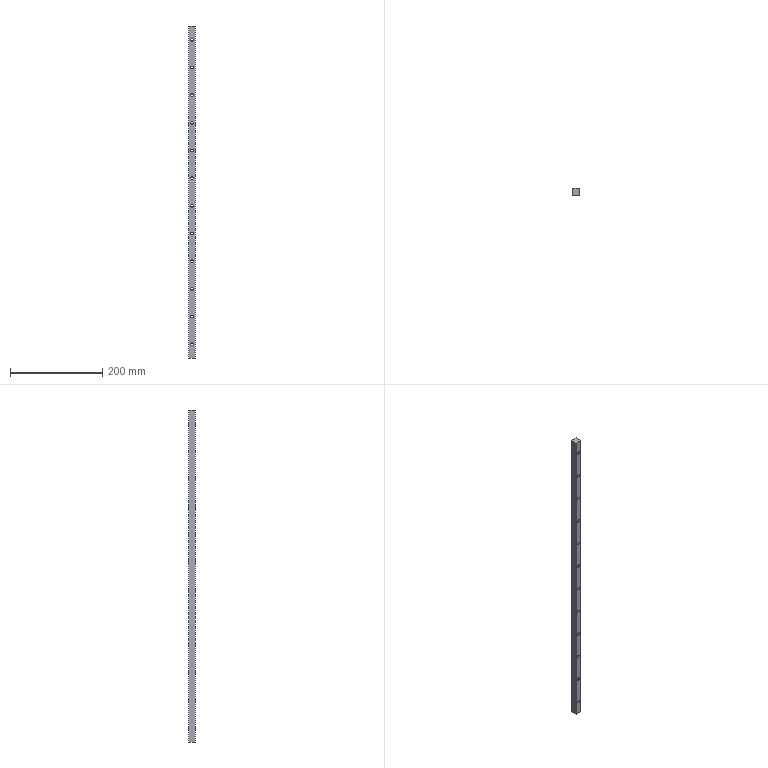Part | 1 solid | 30 faces | box 15 x 15 x 720 mm | volume 156911 mm3 | cylinder 24 | plane 6 | commonest cylinder face diameters 6 x24
STEP:
#1=CARTESIAN_POINT('',(7.5,0.,687.));
#2=VERTEX_POINT('',#1);
#3=CARTESIAN_POINT('',(7.5,0.,693.));
#4=VERTEX_POINT('',#3);
#5=CARTESIAN_POINT('',(7.5,0.,690.));
#6=DIRECTION('',(0.,1.,0.));
#7=DIRECTION('',(0.,0.,1.));
#8=AXIS2_PLACEMENT_3D('',#5,#6,#7);
#9=CIRCLE('',#8,3.);
#10=EDGE_CURVE('',#2,#4,#9,.T.);
#11=ORIENTED_EDGE('',*,*,#10,.F.);
#12=CARTESIAN_POINT('',(7.5,15.,687.));
#13=VERTEX_POINT('',#12);
#14=CARTESIAN_POINT('',(7.5,-35.,687.));
#15=DIRECTION('',(0.,1.,0.));
#16=VECTOR('',#15,1000.);
#17=LINE('',#14,#16);
#18=EDGE_CURVE('',#2,#13,#17,.T.);
#19=ORIENTED_EDGE('',*,*,#18,.T.);
#20=CARTESIAN_POINT('',(7.5,15.,693.));
#21=VERTEX_POINT('',#20);
#22=CARTESIAN_POINT('',(7.5,15.,690.));
#23=DIRECTION('',(0.,1.,0.));
#24=DIRECTION('',(0.,0.,1.));
#25=AXIS2_PLACEMENT_3D('',#22,#23,#24);
#26=CIRCLE('',#25,3.);
#27=EDGE_CURVE('',#13,#21,#26,.T.);
#28=ORIENTED_EDGE('',*,*,#27,.T.);
#29=CARTESIAN_POINT('',(7.5,-35.,693.));
#30=DIRECTION('',(0.,1.,0.));
#31=VECTOR('',#30,1000.);
#32=LINE('',#29,#31);
#33=EDGE_CURVE('',#4,#21,#32,.T.);
#34=ORIENTED_EDGE('',*,*,#33,.F.);
#35=EDGE_LOOP('',(#11,#19,#28,#34));
#36=FACE_OUTER_BOUND('',#35,.T.);
#37=CARTESIAN_POINT('',(7.5,-35.,690.));
#38=DIRECTION('',(0.,1.,0.));
#39=DIRECTION('',(0.,0.,1.));
#40=AXIS2_PLACEMENT_3D('',#37,#38,#39);
#41=CYLINDRICAL_SURFACE('',#40,3.);
#42=ADVANCED_FACE('',(#36),#41,.F.);
#43=CARTESIAN_POINT('',(7.5,0.,627.));
#44=VERTEX_POINT('',#43);
#45=CARTESIAN_POINT('',(7.5,0.,633.));
#46=VERTEX_POINT('',#45);
#47=CARTESIAN_POINT('',(7.5,0.,630.));
#48=DIRECTION('',(0.,1.,0.));
#49=DIRECTION('',(0.,0.,1.));
#50=AXIS2_PLACEMENT_3D('',#47,#48,#49);
#51=CIRCLE('',#50,3.);
#52=EDGE_CURVE('',#44,#46,#51,.T.);
#53=ORIENTED_EDGE('',*,*,#52,.F.);
#54=CARTESIAN_POINT('',(7.5,15.,627.));
#55=VERTEX_POINT('',#54);
#56=CARTESIAN_POINT('',(7.5,-35.,627.));
#57=DIRECTION('',(0.,1.,0.));
#58=VECTOR('',#57,1000.);
#59=LINE('',#56,#58);
#60=EDGE_CURVE('',#44,#55,#59,.T.);
#61=ORIENTED_EDGE('',*,*,#60,.T.);
#62=CARTESIAN_POINT('',(7.5,15.,633.));
#63=VERTEX_POINT('',#62);
#64=CARTESIAN_POINT('',(7.5,15.,630.));
#65=DIRECTION('',(0.,1.,0.));
#66=DIRECTION('',(0.,0.,1.));
#67=AXIS2_PLACEMENT_3D('',#64,#65,#66);
#68=CIRCLE('',#67,3.);
#69=EDGE_CURVE('',#55,#63,#68,.T.);
#70=ORIENTED_EDGE('',*,*,#69,.T.);
#71=CARTESIAN_POINT('',(7.5,-35.,633.));
#72=DIRECTION('',(0.,1.,0.));
#73=VECTOR('',#72,1000.);
#74=LINE('',#71,#73);
#75=EDGE_CURVE('',#46,#63,#74,.T.);
#76=ORIENTED_EDGE('',*,*,#75,.F.);
#77=EDGE_LOOP('',(#53,#61,#70,#76));
#78=FACE_OUTER_BOUND('',#77,.T.);
#79=CARTESIAN_POINT('',(7.5,-35.,630.));
#80=DIRECTION('',(0.,1.,0.));
#81=DIRECTION('',(0.,0.,1.));
#82=AXIS2_PLACEMENT_3D('',#79,#80,#81);
#83=CYLINDRICAL_SURFACE('',#82,3.);
#84=ADVANCED_FACE('',(#78),#83,.F.);
#85=CARTESIAN_POINT('',(7.5,0.,567.));
#86=VERTEX_POINT('',#85);
#87=CARTESIAN_POINT('',(7.5,0.,573.));
#88=VERTEX_POINT('',#87);
#89=CARTESIAN_POINT('',(7.5,0.,570.));
#90=DIRECTION('',(0.,1.,0.));
#91=DIRECTION('',(0.,0.,1.));
#92=AXIS2_PLACEMENT_3D('',#89,#90,#91);
#93=CIRCLE('',#92,3.);
#94=EDGE_CURVE('',#86,#88,#93,.T.);
#95=ORIENTED_EDGE('',*,*,#94,.F.);
#96=CARTESIAN_POINT('',(7.5,15.,567.));
#97=VERTEX_POINT('',#96);
#98=CARTESIAN_POINT('',(7.5,-35.,567.));
#99=DIRECTION('',(0.,1.,0.));
#100=VECTOR('',#99,1000.);
#101=LINE('',#98,#100);
#102=EDGE_CURVE('',#86,#97,#101,.T.);
#103=ORIENTED_EDGE('',*,*,#102,.T.);
#104=CARTESIAN_POINT('',(7.5,15.,573.));
#105=VERTEX_POINT('',#104);
#106=CARTESIAN_POINT('',(7.5,15.,570.));
#107=DIRECTION('',(0.,1.,0.));
#108=DIRECTION('',(0.,0.,1.));
#109=AXIS2_PLACEMENT_3D('',#106,#107,#108);
#110=CIRCLE('',#109,3.);
#111=EDGE_CURVE('',#97,#105,#110,.T.);
#112=ORIENTED_EDGE('',*,*,#111,.T.);
#113=CARTESIAN_POINT('',(7.5,-35.,573.));
#114=DIRECTION('',(0.,1.,0.));
#115=VECTOR('',#114,1000.);
#116=LINE('',#113,#115);
#117=EDGE_CURVE('',#88,#105,#116,.T.);
#118=ORIENTED_EDGE('',*,*,#117,.F.);
#119=EDGE_LOOP('',(#95,#103,#112,#118));
#120=FACE_OUTER_BOUND('',#119,.T.);
#121=CARTESIAN_POINT('',(7.5,-35.,570.));
#122=DIRECTION('',(0.,1.,0.));
#123=DIRECTION('',(0.,0.,1.));
#124=AXIS2_PLACEMENT_3D('',#121,#122,#123);
#125=CYLINDRICAL_SURFACE('',#124,3.);
#126=ADVANCED_FACE('',(#120),#125,.F.);
#127=CARTESIAN_POINT('',(7.5,0.,507.));
#128=VERTEX_POINT('',#127);
#129=CARTESIAN_POINT('',(7.5,0.,513.));
#130=VERTEX_POINT('',#129);
#131=CARTESIAN_POINT('',(7.5,0.,510.));
#132=DIRECTION('',(0.,1.,0.));
#133=DIRECTION('',(0.,0.,1.));
#134=AXIS2_PLACEMENT_3D('',#131,#132,#133);
#135=CIRCLE('',#134,3.);
#136=EDGE_CURVE('',#128,#130,#135,.T.);
#137=ORIENTED_EDGE('',*,*,#136,.F.);
#138=CARTESIAN_POINT('',(7.5,15.,507.));
#139=VERTEX_POINT('',#138);
#140=CARTESIAN_POINT('',(7.5,-35.,507.));
#141=DIRECTION('',(0.,1.,0.));
#142=VECTOR('',#141,1000.);
#143=LINE('',#140,#142);
#144=EDGE_CURVE('',#128,#139,#143,.T.);
#145=ORIENTED_EDGE('',*,*,#144,.T.);
#146=CARTESIAN_POINT('',(7.5,15.,513.));
#147=VERTEX_POINT('',#146);
#148=CARTESIAN_POINT('',(7.5,15.,510.));
#149=DIRECTION('',(0.,1.,0.));
#150=DIRECTION('',(0.,0.,1.));
#151=AXIS2_PLACEMENT_3D('',#148,#149,#150);
#152=CIRCLE('',#151,3.);
#153=EDGE_CURVE('',#139,#147,#152,.T.);
#154=ORIENTED_EDGE('',*,*,#153,.T.);
#155=CARTESIAN_POINT('',(7.5,-35.,513.));
#156=DIRECTION('',(0.,1.,0.));
#157=VECTOR('',#156,1000.);
#158=LINE('',#155,#157);
#159=EDGE_CURVE('',#130,#147,#158,.T.);
#160=ORIENTED_EDGE('',*,*,#159,.F.);
#161=EDGE_LOOP('',(#137,#145,#154,#160));
#162=FACE_OUTER_BOUND('',#161,.T.);
#163=CARTESIAN_POINT('',(7.5,-35.,510.));
#164=DIRECTION('',(0.,1.,0.));
#165=DIRECTION('',(0.,0.,1.));
#166=AXIS2_PLACEMENT_3D('',#163,#164,#165);
#167=CYLINDRICAL_SURFACE('',#166,3.);
#168=ADVANCED_FACE('',(#162),#167,.F.);
#169=CARTESIAN_POINT('',(7.5,0.,447.));
#170=VERTEX_POINT('',#169);
#171=CARTESIAN_POINT('',(7.5,0.,453.));
#172=VERTEX_POINT('',#171);
#173=CARTESIAN_POINT('',(7.5,0.,450.));
#174=DIRECTION('',(0.,1.,0.));
#175=DIRECTION('',(0.,0.,1.));
#176=AXIS2_PLACEMENT_3D('',#173,#174,#175);
#177=CIRCLE('',#176,3.);
#178=EDGE_CURVE('',#170,#172,#177,.T.);
#179=ORIENTED_EDGE('',*,*,#178,.F.);
#180=CARTESIAN_POINT('',(7.5,15.,447.));
#181=VERTEX_POINT('',#180);
#182=CARTESIAN_POINT('',(7.5,-35.,447.));
#183=DIRECTION('',(0.,1.,0.));
#184=VECTOR('',#183,1000.);
#185=LINE('',#182,#184);
#186=EDGE_CURVE('',#170,#181,#185,.T.);
#187=ORIENTED_EDGE('',*,*,#186,.T.);
#188=CARTESIAN_POINT('',(7.5,15.,453.));
#189=VERTEX_POINT('',#188);
#190=CARTESIAN_POINT('',(7.5,15.,450.));
#191=DIRECTION('',(0.,1.,0.));
#192=DIRECTION('',(0.,0.,1.));
#193=AXIS2_PLACEMENT_3D('',#190,#191,#192);
#194=CIRCLE('',#193,3.);
#195=EDGE_CURVE('',#181,#189,#194,.T.);
#196=ORIENTED_EDGE('',*,*,#195,.T.);
#197=CARTESIAN_POINT('',(7.5,-35.,453.));
#198=DIRECTION('',(0.,1.,0.));
#199=VECTOR('',#198,1000.);
#200=LINE('',#197,#199);
#201=EDGE_CURVE('',#172,#189,#200,.T.);
#202=ORIENTED_EDGE('',*,*,#201,.F.);
#203=EDGE_LOOP('',(#179,#187,#196,#202));
#204=FACE_OUTER_BOUND('',#203,.T.);
#205=CARTESIAN_POINT('',(7.5,-35.,450.));
#206=DIRECTION('',(0.,1.,0.));
#207=DIRECTION('',(0.,0.,1.));
#208=AXIS2_PLACEMENT_3D('',#205,#206,#207);
#209=CYLINDRICAL_SURFACE('',#208,3.);
#210=ADVANCED_FACE('',(#204),#209,.F.);
#211=CARTESIAN_POINT('',(7.5,0.,387.));
#212=VERTEX_POINT('',#211);
#213=CARTESIAN_POINT('',(7.5,0.,393.));
#214=VERTEX_POINT('',#213);
#215=CARTESIAN_POINT('',(7.5,0.,390.));
#216=DIRECTION('',(0.,1.,0.));
#217=DIRECTION('',(0.,0.,1.));
#218=AXIS2_PLACEMENT_3D('',#215,#216,#217);
#219=CIRCLE('',#218,3.);
#220=EDGE_CURVE('',#212,#214,#219,.T.);
#221=ORIENTED_EDGE('',*,*,#220,.F.);
#222=CARTESIAN_POINT('',(7.5,15.,387.));
#223=VERTEX_POINT('',#222);
#224=CARTESIAN_POINT('',(7.5,-35.,387.));
#225=DIRECTION('',(0.,1.,0.));
#226=VECTOR('',#225,1000.);
#227=LINE('',#224,#226);
#228=EDGE_CURVE('',#212,#223,#227,.T.);
#229=ORIENTED_EDGE('',*,*,#228,.T.);
#230=CARTESIAN_POINT('',(7.5,15.,393.));
#231=VERTEX_POINT('',#230);
#232=CARTESIAN_POINT('',(7.5,15.,390.));
#233=DIRECTION('',(0.,1.,0.));
#234=DIRECTION('',(0.,0.,1.));
#235=AXIS2_PLACEMENT_3D('',#232,#233,#234);
#236=CIRCLE('',#235,3.);
#237=EDGE_CURVE('',#223,#231,#236,.T.);
#238=ORIENTED_EDGE('',*,*,#237,.T.);
#239=CARTESIAN_POINT('',(7.5,-35.,393.));
#240=DIRECTION('',(0.,1.,0.));
#241=VECTOR('',#240,1000.);
#242=LINE('',#239,#241);
#243=EDGE_CURVE('',#214,#231,#242,.T.);
#244=ORIENTED_EDGE('',*,*,#243,.F.);
#245=EDGE_LOOP('',(#221,#229,#238,#244));
#246=FACE_OUTER_BOUND('',#245,.T.);
#247=CARTESIAN_POINT('',(7.5,-35.,390.));
#248=DIRECTION('',(0.,1.,0.));
#249=DIRECTION('',(0.,0.,1.));
#250=AXIS2_PLACEMENT_3D('',#247,#248,#249);
#251=CYLINDRICAL_SURFACE('',#250,3.);
#252=ADVANCED_FACE('',(#246),#251,.F.);
#253=CARTESIAN_POINT('',(7.5,0.,327.));
#254=VERTEX_POINT('',#253);
#255=CARTESIAN_POINT('',(7.5,0.,333.));
#256=VERTEX_POINT('',#255);
#257=CARTESIAN_POINT('',(7.5,0.,330.));
#258=DIRECTION('',(0.,1.,0.));
#259=DIRECTION('',(0.,0.,1.));
#260=AXIS2_PLACEMENT_3D('',#257,#258,#259);
#261=CIRCLE('',#260,3.);
#262=EDGE_CURVE('',#254,#256,#261,.T.);
#263=ORIENTED_EDGE('',*,*,#262,.F.);
#264=CARTESIAN_POINT('',(7.5,15.,327.));
#265=VERTEX_POINT('',#264);
#266=CARTESIAN_POINT('',(7.5,-35.,327.));
#267=DIRECTION('',(0.,1.,0.));
#268=VECTOR('',#267,1000.);
#269=LINE('',#266,#268);
#270=EDGE_CURVE('',#254,#265,#269,.T.);
#271=ORIENTED_EDGE('',*,*,#270,.T.);
#272=CARTESIAN_POINT('',(7.5,15.,333.));
#273=VERTEX_POINT('',#272);
#274=CARTESIAN_POINT('',(7.5,15.,330.));
#275=DIRECTION('',(0.,1.,0.));
#276=DIRECTION('',(0.,0.,1.));
#277=AXIS2_PLACEMENT_3D('',#274,#275,#276);
#278=CIRCLE('',#277,3.);
#279=EDGE_CURVE('',#265,#273,#278,.T.);
#280=ORIENTED_EDGE('',*,*,#279,.T.);
#281=CARTESIAN_POINT('',(7.5,-35.,333.));
#282=DIRECTION('',(0.,1.,0.));
#283=VECTOR('',#282,1000.);
#284=LINE('',#281,#283);
#285=EDGE_CURVE('',#256,#273,#284,.T.);
#286=ORIENTED_EDGE('',*,*,#285,.F.);
#287=EDGE_LOOP('',(#263,#271,#280,#286));
#288=FACE_OUTER_BOUND('',#287,.T.);
#289=CARTESIAN_POINT('',(7.5,-35.,330.));
#290=DIRECTION('',(0.,1.,0.));
#291=DIRECTION('',(0.,0.,1.));
#292=AXIS2_PLACEMENT_3D('',#289,#290,#291);
#293=CYLINDRICAL_SURFACE('',#292,3.);
#294=ADVANCED_FACE('',(#288),#293,.F.);
#295=CARTESIAN_POINT('',(7.5,0.,267.));
#296=VERTEX_POINT('',#295);
#297=CARTESIAN_POINT('',(7.5,0.,273.));
#298=VERTEX_POINT('',#297);
#299=CARTESIAN_POINT('',(7.5,0.,270.));
#300=DIRECTION('',(0.,1.,0.));
#301=DIRECTION('',(0.,0.,1.));
#302=AXIS2_PLACEMENT_3D('',#299,#300,#301);
#303=CIRCLE('',#302,3.);
#304=EDGE_CURVE('',#296,#298,#303,.T.);
#305=ORIENTED_EDGE('',*,*,#304,.F.);
#306=CARTESIAN_POINT('',(7.5,15.,267.));
#307=VERTEX_POINT('',#306);
#308=CARTESIAN_POINT('',(7.5,-35.,267.));
#309=DIRECTION('',(0.,1.,0.));
#310=VECTOR('',#309,1000.);
#311=LINE('',#308,#310);
#312=EDGE_CURVE('',#296,#307,#311,.T.);
#313=ORIENTED_EDGE('',*,*,#312,.T.);
#314=CARTESIAN_POINT('',(7.5,15.,273.));
#315=VERTEX_POINT('',#314);
#316=CARTESIAN_POINT('',(7.5,15.,270.));
#317=DIRECTION('',(0.,1.,0.));
#318=DIRECTION('',(0.,0.,1.));
#319=AXIS2_PLACEMENT_3D('',#316,#317,#318);
#320=CIRCLE('',#319,3.);
#321=EDGE_CURVE('',#307,#315,#320,.T.);
#322=ORIENTED_EDGE('',*,*,#321,.T.);
#323=CARTESIAN_POINT('',(7.5,-35.,273.));
#324=DIRECTION('',(0.,1.,0.));
#325=VECTOR('',#324,1000.);
#326=LINE('',#323,#325);
#327=EDGE_CURVE('',#298,#315,#326,.T.);
#328=ORIENTED_EDGE('',*,*,#327,.F.);
#329=EDGE_LOOP('',(#305,#313,#322,#328));
#330=FACE_OUTER_BOUND('',#329,.T.);
#331=CARTESIAN_POINT('',(7.5,-35.,270.));
#332=DIRECTION('',(0.,1.,0.));
#333=DIRECTION('',(0.,0.,1.));
#334=AXIS2_PLACEMENT_3D('',#331,#332,#333);
#335=CYLINDRICAL_SURFACE('',#334,3.);
#336=ADVANCED_FACE('',(#330),#335,.F.);
#337=CARTESIAN_POINT('',(7.5,0.,207.));
#338=VERTEX_POINT('',#337);
#339=CARTESIAN_POINT('',(7.5,0.,213.));
#340=VERTEX_POINT('',#339);
#341=CARTESIAN_POINT('',(7.5,0.,210.));
#342=DIRECTION('',(0.,1.,0.));
#343=DIRECTION('',(0.,0.,1.));
#344=AXIS2_PLACEMENT_3D('',#341,#342,#343);
#345=CIRCLE('',#344,3.);
#346=EDGE_CURVE('',#338,#340,#345,.T.);
#347=ORIENTED_EDGE('',*,*,#346,.F.);
#348=CARTESIAN_POINT('',(7.5,15.,207.));
#349=VERTEX_POINT('',#348);
#350=CARTESIAN_POINT('',(7.5,-35.,207.));
#351=DIRECTION('',(0.,1.,0.));
#352=VECTOR('',#351,1000.);
#353=LINE('',#350,#352);
#354=EDGE_CURVE('',#338,#349,#353,.T.);
#355=ORIENTED_EDGE('',*,*,#354,.T.);
#356=CARTESIAN_POINT('',(7.5,15.,213.));
#357=VERTEX_POINT('',#356);
#358=CARTESIAN_POINT('',(7.5,15.,210.));
#359=DIRECTION('',(0.,1.,0.));
#360=DIRECTION('',(0.,0.,1.));
#361=AXIS2_PLACEMENT_3D('',#358,#359,#360);
#362=CIRCLE('',#361,3.);
#363=EDGE_CURVE('',#349,#357,#362,.T.);
#364=ORIENTED_EDGE('',*,*,#363,.T.);
#365=CARTESIAN_POINT('',(7.5,-35.,213.));
#366=DIRECTION('',(0.,1.,0.));
#367=VECTOR('',#366,1000.);
#368=LINE('',#365,#367);
#369=EDGE_CURVE('',#340,#357,#368,.T.);
#370=ORIENTED_EDGE('',*,*,#369,.F.);
#371=EDGE_LOOP('',(#347,#355,#364,#370));
#372=FACE_OUTER_BOUND('',#371,.T.);
#373=CARTESIAN_POINT('',(7.5,-35.,210.));
#374=DIRECTION('',(0.,1.,0.));
#375=DIRECTION('',(0.,0.,1.));
#376=AXIS2_PLACEMENT_3D('',#373,#374,#375);
#377=CYLINDRICAL_SURFACE('',#376,3.);
#378=ADVANCED_FACE('',(#372),#377,.F.);
#379=CARTESIAN_POINT('',(7.5,0.,147.));
#380=VERTEX_POINT('',#379);
#381=CARTESIAN_POINT('',(7.5,0.,153.));
#382=VERTEX_POINT('',#381);
#383=CARTESIAN_POINT('',(7.5,0.,150.));
#384=DIRECTION('',(0.,1.,0.));
#385=DIRECTION('',(0.,0.,1.));
#386=AXIS2_PLACEMENT_3D('',#383,#384,#385);
#387=CIRCLE('',#386,3.);
#388=EDGE_CURVE('',#380,#382,#387,.T.);
#389=ORIENTED_EDGE('',*,*,#388,.F.);
#390=CARTESIAN_POINT('',(7.5,15.,147.));
#391=VERTEX_POINT('',#390);
#392=CARTESIAN_POINT('',(7.5,-35.,147.));
#393=DIRECTION('',(0.,1.,0.));
#394=VECTOR('',#393,1000.);
#395=LINE('',#392,#394);
#396=EDGE_CURVE('',#380,#391,#395,.T.);
#397=ORIENTED_EDGE('',*,*,#396,.T.);
#398=CARTESIAN_POINT('',(7.5,15.,153.));
#399=VERTEX_POINT('',#398);
#400=CARTESIAN_POINT('',(7.5,15.,150.));
#401=DIRECTION('',(0.,1.,0.));
#402=DIRECTION('',(0.,0.,1.));
#403=AXIS2_PLACEMENT_3D('',#400,#401,#402);
#404=CIRCLE('',#403,3.);
#405=EDGE_CURVE('',#391,#399,#404,.T.);
#406=ORIENTED_EDGE('',*,*,#405,.T.);
#407=CARTESIAN_POINT('',(7.5,-35.,153.));
#408=DIRECTION('',(0.,1.,0.));
#409=VECTOR('',#408,1000.);
#410=LINE('',#407,#409);
#411=EDGE_CURVE('',#382,#399,#410,.T.);
#412=ORIENTED_EDGE('',*,*,#411,.F.);
#413=EDGE_LOOP('',(#389,#397,#406,#412));
#414=FACE_OUTER_BOUND('',#413,.T.);
#415=CARTESIAN_POINT('',(7.5,-35.,150.));
#416=DIRECTION('',(0.,1.,0.));
#417=DIRECTION('',(0.,0.,1.));
#418=AXIS2_PLACEMENT_3D('',#415,#416,#417);
#419=CYLINDRICAL_SURFACE('',#418,3.);
#420=ADVANCED_FACE('',(#414),#419,.F.);
#421=CARTESIAN_POINT('',(7.5,0.,87.));
#422=VERTEX_POINT('',#421);
#423=CARTESIAN_POINT('',(7.5,0.,93.));
#424=VERTEX_POINT('',#423);
#425=CARTESIAN_POINT('',(7.5,0.,90.));
#426=DIRECTION('',(0.,1.,0.));
#427=DIRECTION('',(0.,0.,1.));
#428=AXIS2_PLACEMENT_3D('',#425,#426,#427);
#429=CIRCLE('',#428,3.);
#430=EDGE_CURVE('',#422,#424,#429,.T.);
#431=ORIENTED_EDGE('',*,*,#430,.F.);
#432=CARTESIAN_POINT('',(7.5,15.,87.));
#433=VERTEX_POINT('',#432);
#434=CARTESIAN_POINT('',(7.5,-35.,87.));
#435=DIRECTION('',(0.,1.,0.));
#436=VECTOR('',#435,1000.);
#437=LINE('',#434,#436);
#438=EDGE_CURVE('',#422,#433,#437,.T.);
#439=ORIENTED_EDGE('',*,*,#438,.T.);
#440=CARTESIAN_POINT('',(7.5,15.,93.));
#441=VERTEX_POINT('',#440);
#442=CARTESIAN_POINT('',(7.5,15.,90.));
#443=DIRECTION('',(0.,1.,0.));
#444=DIRECTION('',(0.,0.,1.));
#445=AXIS2_PLACEMENT_3D('',#442,#443,#444);
#446=CIRCLE('',#445,3.);
#447=EDGE_CURVE('',#433,#441,#446,.T.);
#448=ORIENTED_EDGE('',*,*,#447,.T.);
#449=CARTESIAN_POINT('',(7.5,-35.,93.));
#450=DIRECTION('',(0.,1.,0.));
#451=VECTOR('',#450,1000.);
#452=LINE('',#449,#451);
#453=EDGE_CURVE('',#424,#441,#452,.T.);
#454=ORIENTED_EDGE('',*,*,#453,.F.);
#455=EDGE_LOOP('',(#431,#439,#448,#454));
#456=FACE_OUTER_BOUND('',#455,.T.);
#457=CARTESIAN_POINT('',(7.5,-35.,90.));
#458=DIRECTION('',(0.,1.,0.));
#459=DIRECTION('',(0.,0.,1.));
#460=AXIS2_PLACEMENT_3D('',#457,#458,#459);
#461=CYLINDRICAL_SURFACE('',#460,3.);
#462=ADVANCED_FACE('',(#456),#461,.F.);
#463=CARTESIAN_POINT('',(7.5,0.,27.));
#464=VERTEX_POINT('',#463);
#465=CARTESIAN_POINT('',(7.5,0.,33.));
#466=VERTEX_POINT('',#465);
#467=CARTESIAN_POINT('',(7.5,0.,30.));
#468=DIRECTION('',(0.,1.,0.));
#469=DIRECTION('',(0.,0.,1.));
#470=AXIS2_PLACEMENT_3D('',#467,#468,#469);
#471=CIRCLE('',#470,3.);
#472=EDGE_CURVE('',#464,#466,#471,.T.);
#473=ORIENTED_EDGE('',*,*,#472,.F.);
#474=CARTESIAN_POINT('',(7.5,15.,27.));
#475=VERTEX_POINT('',#474);
#476=CARTESIAN_POINT('',(7.5,-35.,27.));
#477=DIRECTION('',(0.,1.,0.));
#478=VECTOR('',#477,1000.);
#479=LINE('',#476,#478);
#480=EDGE_CURVE('',#464,#475,#479,.T.);
#481=ORIENTED_EDGE('',*,*,#480,.T.);
#482=CARTESIAN_POINT('',(7.5,15.,33.));
#483=VERTEX_POINT('',#482);
#484=CARTESIAN_POINT('',(7.5,15.,30.));
#485=DIRECTION('',(0.,1.,0.));
#486=DIRECTION('',(0.,0.,1.));
#487=AXIS2_PLACEMENT_3D('',#484,#485,#486);
#488=CIRCLE('',#487,3.);
#489=EDGE_CURVE('',#475,#483,#488,.T.);
#490=ORIENTED_EDGE('',*,*,#489,.T.);
#491=CARTESIAN_POINT('',(7.5,-35.,33.));
#492=DIRECTION('',(0.,1.,0.));
#493=VECTOR('',#492,1000.);
#494=LINE('',#491,#493);
#495=EDGE_CURVE('',#466,#483,#494,.T.);
#496=ORIENTED_EDGE('',*,*,#495,.F.);
#497=EDGE_LOOP('',(#473,#481,#490,#496));
#498=FACE_OUTER_BOUND('',#497,.T.);
#499=CARTESIAN_POINT('',(7.5,-35.,30.));
#500=DIRECTION('',(0.,1.,0.));
#501=DIRECTION('',(0.,0.,1.));
#502=AXIS2_PLACEMENT_3D('',#499,#500,#501);
#503=CYLINDRICAL_SURFACE('',#502,3.);
#504=ADVANCED_FACE('',(#498),#503,.F.);
#505=CARTESIAN_POINT('',(0.,15.,0.));
#506=VERTEX_POINT('',#505);
#507=CARTESIAN_POINT('',(0.,0.,0.));
#508=VERTEX_POINT('',#507);
#509=CARTESIAN_POINT('',(0.,0.,0.));
#510=DIRECTION('',(0.,-1.,0.));
#511=VECTOR('',#510,1000.);
#512=LINE('',#509,#511);
#513=EDGE_CURVE('',#506,#508,#512,.T.);
#514=ORIENTED_EDGE('',*,*,#513,.T.);
#515=CARTESIAN_POINT('',(0.,0.,720.));
#516=VERTEX_POINT('',#515);
#517=CARTESIAN_POINT('',(0.,0.,720.));
#518=DIRECTION('',(0.,0.,-1.));
#519=VECTOR('',#518,1000.);
#520=LINE('',#517,#519);
#521=EDGE_CURVE('',#516,#508,#520,.T.);
#522=ORIENTED_EDGE('',*,*,#521,.F.);
#523=CARTESIAN_POINT('',(0.,15.,720.));
#524=VERTEX_POINT('',#523);
#525=CARTESIAN_POINT('',(0.,0.,720.));
#526=DIRECTION('',(0.,-1.,0.));
#527=VECTOR('',#526,1000.);
#528=LINE('',#525,#527);
#529=EDGE_CURVE('',#524,#516,#528,.T.);
#530=ORIENTED_EDGE('',*,*,#529,.F.);
#531=CARTESIAN_POINT('',(0.,15.,720.));
#532=DIRECTION('',(0.,0.,-1.));
#533=VECTOR('',#532,1000.);
#534=LINE('',#531,#533);
#535=EDGE_CURVE('',#524,#506,#534,.T.);
#536=ORIENTED_EDGE('',*,*,#535,.T.);
#537=EDGE_LOOP('',(#514,#522,#530,#536));
#538=FACE_OUTER_BOUND('',#537,.T.);
#539=CARTESIAN_POINT('',(0.,0.,720.));
#540=DIRECTION('',(1.,0.,0.));
#541=DIRECTION('',(0.,0.,-1.));
#542=AXIS2_PLACEMENT_3D('',#539,#540,#541);
#543=PLANE('',#542);
#544=ADVANCED_FACE('',(#538),#543,.F.);
#545=CARTESIAN_POINT('',(7.5,0.,90.));
#546=DIRECTION('',(0.,1.,0.));
#547=DIRECTION('',(0.,0.,1.));
#548=AXIS2_PLACEMENT_3D('',#545,#546,#547);
#549=CIRCLE('',#548,3.);
#550=EDGE_CURVE('',#424,#422,#549,.T.);
#551=ORIENTED_EDGE('',*,*,#550,.T.);
#552=ORIENTED_EDGE('',*,*,#430,.T.);
#553=EDGE_LOOP('',(#551,#552));
#554=FACE_BOUND('',#553,.T.);
#555=CARTESIAN_POINT('',(7.5,0.,30.));
#556=DIRECTION('',(0.,1.,0.));
#557=DIRECTION('',(0.,0.,1.));
#558=AXIS2_PLACEMENT_3D('',#555,#556,#557);
#559=CIRCLE('',#558,3.);
#560=EDGE_CURVE('',#466,#464,#559,.T.);
#561=ORIENTED_EDGE('',*,*,#560,.T.);
#562=ORIENTED_EDGE('',*,*,#472,.T.);
#563=EDGE_LOOP('',(#561,#562));
#564=FACE_BOUND('',#563,.T.);
#565=CARTESIAN_POINT('',(15.,0.,0.));
#566=VERTEX_POINT('',#565);
#567=CARTESIAN_POINT('',(0.,0.,0.));
#568=DIRECTION('',(1.,0.,0.));
#569=VECTOR('',#568,1000.);
#570=LINE('',#567,#569);
#571=EDGE_CURVE('',#508,#566,#570,.T.);
#572=ORIENTED_EDGE('',*,*,#571,.T.);
#573=CARTESIAN_POINT('',(15.,0.,720.));
#574=VERTEX_POINT('',#573);
#575=CARTESIAN_POINT('',(15.,0.,720.));
#576=DIRECTION('',(0.,0.,-1.));
#577=VECTOR('',#576,1000.);
#578=LINE('',#575,#577);
#579=EDGE_CURVE('',#574,#566,#578,.T.);
#580=ORIENTED_EDGE('',*,*,#579,.F.);
#581=CARTESIAN_POINT('',(0.,0.,720.));
#582=DIRECTION('',(1.,0.,0.));
#583=VECTOR('',#582,1000.);
#584=LINE('',#581,#583);
#585=EDGE_CURVE('',#516,#574,#584,.T.);
#586=ORIENTED_EDGE('',*,*,#585,.F.);
#587=ORIENTED_EDGE('',*,*,#521,.T.);
#588=EDGE_LOOP('',(#572,#580,#586,#587));
#589=FACE_OUTER_BOUND('',#588,.T.);
#590=CARTESIAN_POINT('',(7.5,0.,150.));
#591=DIRECTION('',(0.,1.,0.));
#592=DIRECTION('',(0.,0.,1.));
#593=AXIS2_PLACEMENT_3D('',#590,#591,#592);
#594=CIRCLE('',#593,3.);
#595=EDGE_CURVE('',#382,#380,#594,.T.);
#596=ORIENTED_EDGE('',*,*,#595,.T.);
#597=ORIENTED_EDGE('',*,*,#388,.T.);
#598=EDGE_LOOP('',(#596,#597));
#599=FACE_BOUND('',#598,.T.);
#600=CARTESIAN_POINT('',(7.5,0.,210.));
#601=DIRECTION('',(0.,1.,0.));
#602=DIRECTION('',(0.,0.,1.));
#603=AXIS2_PLACEMENT_3D('',#600,#601,#602);
#604=CIRCLE('',#603,3.);
#605=EDGE_CURVE('',#340,#338,#604,.T.);
#606=ORIENTED_EDGE('',*,*,#605,.T.);
#607=ORIENTED_EDGE('',*,*,#346,.T.);
#608=EDGE_LOOP('',(#606,#607));
#609=FACE_BOUND('',#608,.T.);
#610=CARTESIAN_POINT('',(7.5,0.,270.));
#611=DIRECTION('',(0.,1.,0.));
#612=DIRECTION('',(0.,0.,1.));
#613=AXIS2_PLACEMENT_3D('',#610,#611,#612);
#614=CIRCLE('',#613,3.);
#615=EDGE_CURVE('',#298,#296,#614,.T.);
#616=ORIENTED_EDGE('',*,*,#615,.T.);
#617=ORIENTED_EDGE('',*,*,#304,.T.);
#618=EDGE_LOOP('',(#616,#617));
#619=FACE_BOUND('',#618,.T.);
#620=CARTESIAN_POINT('',(7.5,0.,330.));
#621=DIRECTION('',(0.,1.,0.));
#622=DIRECTION('',(0.,0.,1.));
#623=AXIS2_PLACEMENT_3D('',#620,#621,#622);
#624=CIRCLE('',#623,3.);
#625=EDGE_CURVE('',#256,#254,#624,.T.);
#626=ORIENTED_EDGE('',*,*,#625,.T.);
#627=ORIENTED_EDGE('',*,*,#262,.T.);
#628=EDGE_LOOP('',(#626,#627));
#629=FACE_BOUND('',#628,.T.);
#630=CARTESIAN_POINT('',(7.5,0.,390.));
#631=DIRECTION('',(0.,1.,0.));
#632=DIRECTION('',(0.,0.,1.));
#633=AXIS2_PLACEMENT_3D('',#630,#631,#632);
#634=CIRCLE('',#633,3.);
#635=EDGE_CURVE('',#214,#212,#634,.T.);
#636=ORIENTED_EDGE('',*,*,#635,.T.);
#637=ORIENTED_EDGE('',*,*,#220,.T.);
#638=EDGE_LOOP('',(#636,#637));
#639=FACE_BOUND('',#638,.T.);
#640=CARTESIAN_POINT('',(7.5,0.,450.));
#641=DIRECTION('',(0.,1.,0.));
#642=DIRECTION('',(0.,0.,1.));
#643=AXIS2_PLACEMENT_3D('',#640,#641,#642);
#644=CIRCLE('',#643,3.);
#645=EDGE_CURVE('',#172,#170,#644,.T.);
#646=ORIENTED_EDGE('',*,*,#645,.T.);
#647=ORIENTED_EDGE('',*,*,#178,.T.);
#648=EDGE_LOOP('',(#646,#647));
#649=FACE_BOUND('',#648,.T.);
#650=CARTESIAN_POINT('',(7.5,0.,510.));
#651=DIRECTION('',(0.,1.,0.));
#652=DIRECTION('',(0.,0.,1.));
#653=AXIS2_PLACEMENT_3D('',#650,#651,#652);
#654=CIRCLE('',#653,3.);
#655=EDGE_CURVE('',#130,#128,#654,.T.);
#656=ORIENTED_EDGE('',*,*,#655,.T.);
#657=ORIENTED_EDGE('',*,*,#136,.T.);
#658=EDGE_LOOP('',(#656,#657));
#659=FACE_BOUND('',#658,.T.);
#660=CARTESIAN_POINT('',(7.5,0.,570.));
#661=DIRECTION('',(0.,1.,0.));
#662=DIRECTION('',(0.,0.,1.));
#663=AXIS2_PLACEMENT_3D('',#660,#661,#662);
#664=CIRCLE('',#663,3.);
#665=EDGE_CURVE('',#88,#86,#664,.T.);
#666=ORIENTED_EDGE('',*,*,#665,.T.);
#667=ORIENTED_EDGE('',*,*,#94,.T.);
#668=EDGE_LOOP('',(#666,#667));
#669=FACE_BOUND('',#668,.T.);
#670=CARTESIAN_POINT('',(7.5,0.,630.));
#671=DIRECTION('',(0.,1.,0.));
#672=DIRECTION('',(0.,0.,1.));
#673=AXIS2_PLACEMENT_3D('',#670,#671,#672);
#674=CIRCLE('',#673,3.);
#675=EDGE_CURVE('',#46,#44,#674,.T.);
#676=ORIENTED_EDGE('',*,*,#675,.T.);
#677=ORIENTED_EDGE('',*,*,#52,.T.);
#678=EDGE_LOOP('',(#676,#677));
#679=FACE_BOUND('',#678,.T.);
#680=CARTESIAN_POINT('',(7.5,0.,690.));
#681=DIRECTION('',(0.,1.,0.));
#682=DIRECTION('',(0.,0.,1.));
#683=AXIS2_PLACEMENT_3D('',#680,#681,#682);
#684=CIRCLE('',#683,3.);
#685=EDGE_CURVE('',#4,#2,#684,.T.);
#686=ORIENTED_EDGE('',*,*,#685,.T.);
#687=ORIENTED_EDGE('',*,*,#10,.T.);
#688=EDGE_LOOP('',(#686,#687));
#689=FACE_BOUND('',#688,.T.);
#690=CARTESIAN_POINT('',(0.,0.,720.));
#691=DIRECTION('',(0.,1.,0.));
#692=DIRECTION('',(0.,0.,1.));
#693=AXIS2_PLACEMENT_3D('',#690,#691,#692);
#694=PLANE('',#693);
#695=ADVANCED_FACE('',(#554,#564,#589,#599,#609,#619,#629,#639,#649,#659,#669,#679,#689),#694,.F.);
#696=CARTESIAN_POINT('',(15.,15.,0.));
#697=VERTEX_POINT('',#696);
#698=CARTESIAN_POINT('',(15.,0.,0.));
#699=DIRECTION('',(0.,1.,0.));
#700=VECTOR('',#699,1000.);
#701=LINE('',#698,#700);
#702=EDGE_CURVE('',#566,#697,#701,.T.);
#703=ORIENTED_EDGE('',*,*,#702,.T.);
#704=CARTESIAN_POINT('',(15.,15.,720.));
#705=VERTEX_POINT('',#704);
#706=CARTESIAN_POINT('',(15.,15.,720.));
#707=DIRECTION('',(0.,0.,-1.));
#708=VECTOR('',#707,1000.);
#709=LINE('',#706,#708);
#710=EDGE_CURVE('',#705,#697,#709,.T.);
#711=ORIENTED_EDGE('',*,*,#710,.F.);
#712=CARTESIAN_POINT('',(15.,0.,720.));
#713=DIRECTION('',(0.,1.,0.));
#714=VECTOR('',#713,1000.);
#715=LINE('',#712,#714);
#716=EDGE_CURVE('',#574,#705,#715,.T.);
#717=ORIENTED_EDGE('',*,*,#716,.F.);
#718=ORIENTED_EDGE('',*,*,#579,.T.);
#719=EDGE_LOOP('',(#703,#711,#717,#718));
#720=FACE_OUTER_BOUND('',#719,.T.);
#721=CARTESIAN_POINT('',(15.,0.,720.));
#722=DIRECTION('',(-1.,0.,0.));
#723=DIRECTION('',(0.,0.,1.));
#724=AXIS2_PLACEMENT_3D('',#721,#722,#723);
#725=PLANE('',#724);
#726=ADVANCED_FACE('',(#720),#725,.F.);
#727=CARTESIAN_POINT('',(7.5,15.,90.));
#728=DIRECTION('',(0.,1.,0.));
#729=DIRECTION('',(0.,0.,1.));
#730=AXIS2_PLACEMENT_3D('',#727,#728,#729);
#731=CIRCLE('',#730,3.);
#732=EDGE_CURVE('',#441,#433,#731,.T.);
#733=ORIENTED_EDGE('',*,*,#732,.F.);
#734=ORIENTED_EDGE('',*,*,#447,.F.);
#735=EDGE_LOOP('',(#733,#734));
#736=FACE_BOUND('',#735,.T.);
#737=CARTESIAN_POINT('',(7.5,15.,30.));
#738=DIRECTION('',(0.,1.,0.));
#739=DIRECTION('',(0.,0.,1.));
#740=AXIS2_PLACEMENT_3D('',#737,#738,#739);
#741=CIRCLE('',#740,3.);
#742=EDGE_CURVE('',#483,#475,#741,.T.);
#743=ORIENTED_EDGE('',*,*,#742,.F.);
#744=ORIENTED_EDGE('',*,*,#489,.F.);
#745=EDGE_LOOP('',(#743,#744));
#746=FACE_BOUND('',#745,.T.);
#747=CARTESIAN_POINT('',(0.,15.,0.));
#748=DIRECTION('',(-1.,0.,0.));
#749=VECTOR('',#748,1000.);
#750=LINE('',#747,#749);
#751=EDGE_CURVE('',#697,#506,#750,.T.);
#752=ORIENTED_EDGE('',*,*,#751,.T.);
#753=ORIENTED_EDGE('',*,*,#535,.F.);
#754=CARTESIAN_POINT('',(0.,15.,720.));
#755=DIRECTION('',(-1.,0.,0.));
#756=VECTOR('',#755,1000.);
#757=LINE('',#754,#756);
#758=EDGE_CURVE('',#705,#524,#757,.T.);
#759=ORIENTED_EDGE('',*,*,#758,.F.);
#760=ORIENTED_EDGE('',*,*,#710,.T.);
#761=EDGE_LOOP('',(#752,#753,#759,#760));
#762=FACE_OUTER_BOUND('',#761,.T.);
#763=CARTESIAN_POINT('',(7.5,15.,150.));
#764=DIRECTION('',(0.,1.,0.));
#765=DIRECTION('',(0.,0.,1.));
#766=AXIS2_PLACEMENT_3D('',#763,#764,#765);
#767=CIRCLE('',#766,3.);
#768=EDGE_CURVE('',#399,#391,#767,.T.);
#769=ORIENTED_EDGE('',*,*,#768,.F.);
#770=ORIENTED_EDGE('',*,*,#405,.F.);
#771=EDGE_LOOP('',(#769,#770));
#772=FACE_BOUND('',#771,.T.);
#773=CARTESIAN_POINT('',(7.5,15.,210.));
#774=DIRECTION('',(0.,1.,0.));
#775=DIRECTION('',(0.,0.,1.));
#776=AXIS2_PLACEMENT_3D('',#773,#774,#775);
#777=CIRCLE('',#776,3.);
#778=EDGE_CURVE('',#357,#349,#777,.T.);
#779=ORIENTED_EDGE('',*,*,#778,.F.);
#780=ORIENTED_EDGE('',*,*,#363,.F.);
#781=EDGE_LOOP('',(#779,#780));
#782=FACE_BOUND('',#781,.T.);
#783=CARTESIAN_POINT('',(7.5,15.,270.));
#784=DIRECTION('',(0.,1.,0.));
#785=DIRECTION('',(0.,0.,1.));
#786=AXIS2_PLACEMENT_3D('',#783,#784,#785);
#787=CIRCLE('',#786,3.);
#788=EDGE_CURVE('',#315,#307,#787,.T.);
#789=ORIENTED_EDGE('',*,*,#788,.F.);
#790=ORIENTED_EDGE('',*,*,#321,.F.);
#791=EDGE_LOOP('',(#789,#790));
#792=FACE_BOUND('',#791,.T.);
#793=CARTESIAN_POINT('',(7.5,15.,330.));
#794=DIRECTION('',(0.,1.,0.));
#795=DIRECTION('',(0.,0.,1.));
#796=AXIS2_PLACEMENT_3D('',#793,#794,#795);
#797=CIRCLE('',#796,3.);
#798=EDGE_CURVE('',#273,#265,#797,.T.);
#799=ORIENTED_EDGE('',*,*,#798,.F.);
#800=ORIENTED_EDGE('',*,*,#279,.F.);
#801=EDGE_LOOP('',(#799,#800));
#802=FACE_BOUND('',#801,.T.);
#803=CARTESIAN_POINT('',(7.5,15.,390.));
#804=DIRECTION('',(0.,1.,0.));
#805=DIRECTION('',(0.,0.,1.));
#806=AXIS2_PLACEMENT_3D('',#803,#804,#805);
#807=CIRCLE('',#806,3.);
#808=EDGE_CURVE('',#231,#223,#807,.T.);
#809=ORIENTED_EDGE('',*,*,#808,.F.);
#810=ORIENTED_EDGE('',*,*,#237,.F.);
#811=EDGE_LOOP('',(#809,#810));
#812=FACE_BOUND('',#811,.T.);
#813=CARTESIAN_POINT('',(7.5,15.,450.));
#814=DIRECTION('',(0.,1.,0.));
#815=DIRECTION('',(0.,0.,1.));
#816=AXIS2_PLACEMENT_3D('',#813,#814,#815);
#817=CIRCLE('',#816,3.);
#818=EDGE_CURVE('',#189,#181,#817,.T.);
#819=ORIENTED_EDGE('',*,*,#818,.F.);
#820=ORIENTED_EDGE('',*,*,#195,.F.);
#821=EDGE_LOOP('',(#819,#820));
#822=FACE_BOUND('',#821,.T.);
#823=CARTESIAN_POINT('',(7.5,15.,510.));
#824=DIRECTION('',(0.,1.,0.));
#825=DIRECTION('',(0.,0.,1.));
#826=AXIS2_PLACEMENT_3D('',#823,#824,#825);
#827=CIRCLE('',#826,3.);
#828=EDGE_CURVE('',#147,#139,#827,.T.);
#829=ORIENTED_EDGE('',*,*,#828,.F.);
#830=ORIENTED_EDGE('',*,*,#153,.F.);
#831=EDGE_LOOP('',(#829,#830));
#832=FACE_BOUND('',#831,.T.);
#833=CARTESIAN_POINT('',(7.5,15.,570.));
#834=DIRECTION('',(0.,1.,0.));
#835=DIRECTION('',(0.,0.,1.));
#836=AXIS2_PLACEMENT_3D('',#833,#834,#835);
#837=CIRCLE('',#836,3.);
#838=EDGE_CURVE('',#105,#97,#837,.T.);
#839=ORIENTED_EDGE('',*,*,#838,.F.);
#840=ORIENTED_EDGE('',*,*,#111,.F.);
#841=EDGE_LOOP('',(#839,#840));
#842=FACE_BOUND('',#841,.T.);
#843=CARTESIAN_POINT('',(7.5,15.,630.));
#844=DIRECTION('',(0.,1.,0.));
#845=DIRECTION('',(0.,0.,1.));
#846=AXIS2_PLACEMENT_3D('',#843,#844,#845);
#847=CIRCLE('',#846,3.);
#848=EDGE_CURVE('',#63,#55,#847,.T.);
#849=ORIENTED_EDGE('',*,*,#848,.F.);
#850=ORIENTED_EDGE('',*,*,#69,.F.);
#851=EDGE_LOOP('',(#849,#850));
#852=FACE_BOUND('',#851,.T.);
#853=CARTESIAN_POINT('',(7.5,15.,690.));
#854=DIRECTION('',(0.,1.,0.));
#855=DIRECTION('',(0.,0.,1.));
#856=AXIS2_PLACEMENT_3D('',#853,#854,#855);
#857=CIRCLE('',#856,3.);
#858=EDGE_CURVE('',#21,#13,#857,.T.);
#859=ORIENTED_EDGE('',*,*,#858,.F.);
#860=ORIENTED_EDGE('',*,*,#27,.F.);
#861=EDGE_LOOP('',(#859,#860));
#862=FACE_BOUND('',#861,.T.);
#863=CARTESIAN_POINT('',(0.,15.,720.));
#864=DIRECTION('',(0.,-1.,0.));
#865=DIRECTION('',(0.,0.,-1.));
#866=AXIS2_PLACEMENT_3D('',#863,#864,#865);
#867=PLANE('',#866);
#868=ADVANCED_FACE('',(#736,#746,#762,#772,#782,#792,#802,#812,#822,#832,#842,#852,#862),#867,.F.);
#869=ORIENTED_EDGE('',*,*,#529,.T.);
#870=ORIENTED_EDGE('',*,*,#585,.T.);
#871=ORIENTED_EDGE('',*,*,#716,.T.);
#872=ORIENTED_EDGE('',*,*,#758,.T.);
#873=EDGE_LOOP('',(#869,#870,#871,#872));
#874=FACE_OUTER_BOUND('',#873,.T.);
#875=CARTESIAN_POINT('',(0.,0.,720.));
#876=DIRECTION('',(0.,0.,-1.));
#877=DIRECTION('',(-1.,0.,0.));
#878=AXIS2_PLACEMENT_3D('',#875,#876,#877);
#879=PLANE('',#878);
#880=ADVANCED_FACE('',(#874),#879,.F.);
#881=ORIENTED_EDGE('',*,*,#513,.F.);
#882=ORIENTED_EDGE('',*,*,#751,.F.);
#883=ORIENTED_EDGE('',*,*,#702,.F.);
#884=ORIENTED_EDGE('',*,*,#571,.F.);
#885=EDGE_LOOP('',(#881,#882,#883,#884));
#886=FACE_OUTER_BOUND('',#885,.T.);
#887=CARTESIAN_POINT('',(0.,0.,0.));
#888=DIRECTION('',(0.,0.,-1.));
#889=DIRECTION('',(-1.,0.,0.));
#890=AXIS2_PLACEMENT_3D('',#887,#888,#889);
#891=PLANE('',#890);
#892=ADVANCED_FACE('',(#886),#891,.T.);
#893=ORIENTED_EDGE('',*,*,#480,.F.);
#894=ORIENTED_EDGE('',*,*,#560,.F.);
#895=ORIENTED_EDGE('',*,*,#495,.T.);
#896=ORIENTED_EDGE('',*,*,#742,.T.);
#897=EDGE_LOOP('',(#893,#894,#895,#896));
#898=FACE_OUTER_BOUND('',#897,.T.);
#899=CARTESIAN_POINT('',(7.5,-35.,30.));
#900=DIRECTION('',(0.,1.,0.));
#901=DIRECTION('',(0.,0.,1.));
#902=AXIS2_PLACEMENT_3D('',#899,#900,#901);
#903=CYLINDRICAL_SURFACE('',#902,3.);
#904=ADVANCED_FACE('',(#898),#903,.F.);
#905=ORIENTED_EDGE('',*,*,#438,.F.);
#906=ORIENTED_EDGE('',*,*,#550,.F.);
#907=ORIENTED_EDGE('',*,*,#453,.T.);
#908=ORIENTED_EDGE('',*,*,#732,.T.);
#909=EDGE_LOOP('',(#905,#906,#907,#908));
#910=FACE_OUTER_BOUND('',#909,.T.);
#911=CARTESIAN_POINT('',(7.5,-35.,90.));
#912=DIRECTION('',(0.,1.,0.));
#913=DIRECTION('',(0.,0.,1.));
#914=AXIS2_PLACEMENT_3D('',#911,#912,#913);
#915=CYLINDRICAL_SURFACE('',#914,3.);
#916=ADVANCED_FACE('',(#910),#915,.F.);
#917=ORIENTED_EDGE('',*,*,#396,.F.);
#918=ORIENTED_EDGE('',*,*,#595,.F.);
#919=ORIENTED_EDGE('',*,*,#411,.T.);
#920=ORIENTED_EDGE('',*,*,#768,.T.);
#921=EDGE_LOOP('',(#917,#918,#919,#920));
#922=FACE_OUTER_BOUND('',#921,.T.);
#923=CARTESIAN_POINT('',(7.5,-35.,150.));
#924=DIRECTION('',(0.,1.,0.));
#925=DIRECTION('',(0.,0.,1.));
#926=AXIS2_PLACEMENT_3D('',#923,#924,#925);
#927=CYLINDRICAL_SURFACE('',#926,3.);
#928=ADVANCED_FACE('',(#922),#927,.F.);
#929=ORIENTED_EDGE('',*,*,#354,.F.);
#930=ORIENTED_EDGE('',*,*,#605,.F.);
#931=ORIENTED_EDGE('',*,*,#369,.T.);
#932=ORIENTED_EDGE('',*,*,#778,.T.);
#933=EDGE_LOOP('',(#929,#930,#931,#932));
#934=FACE_OUTER_BOUND('',#933,.T.);
#935=CARTESIAN_POINT('',(7.5,-35.,210.));
#936=DIRECTION('',(0.,1.,0.));
#937=DIRECTION('',(0.,0.,1.));
#938=AXIS2_PLACEMENT_3D('',#935,#936,#937);
#939=CYLINDRICAL_SURFACE('',#938,3.);
#940=ADVANCED_FACE('',(#934),#939,.F.);
#941=ORIENTED_EDGE('',*,*,#312,.F.);
#942=ORIENTED_EDGE('',*,*,#615,.F.);
#943=ORIENTED_EDGE('',*,*,#327,.T.);
#944=ORIENTED_EDGE('',*,*,#788,.T.);
#945=EDGE_LOOP('',(#941,#942,#943,#944));
#946=FACE_OUTER_BOUND('',#945,.T.);
#947=CARTESIAN_POINT('',(7.5,-35.,270.));
#948=DIRECTION('',(0.,1.,0.));
#949=DIRECTION('',(0.,0.,1.));
#950=AXIS2_PLACEMENT_3D('',#947,#948,#949);
#951=CYLINDRICAL_SURFACE('',#950,3.);
#952=ADVANCED_FACE('',(#946),#951,.F.);
#953=ORIENTED_EDGE('',*,*,#270,.F.);
#954=ORIENTED_EDGE('',*,*,#625,.F.);
#955=ORIENTED_EDGE('',*,*,#285,.T.);
#956=ORIENTED_EDGE('',*,*,#798,.T.);
#957=EDGE_LOOP('',(#953,#954,#955,#956));
#958=FACE_OUTER_BOUND('',#957,.T.);
#959=CARTESIAN_POINT('',(7.5,-35.,330.));
#960=DIRECTION('',(0.,1.,0.));
#961=DIRECTION('',(0.,0.,1.));
#962=AXIS2_PLACEMENT_3D('',#959,#960,#961);
#963=CYLINDRICAL_SURFACE('',#962,3.);
#964=ADVANCED_FACE('',(#958),#963,.F.);
#965=ORIENTED_EDGE('',*,*,#228,.F.);
#966=ORIENTED_EDGE('',*,*,#635,.F.);
#967=ORIENTED_EDGE('',*,*,#243,.T.);
#968=ORIENTED_EDGE('',*,*,#808,.T.);
#969=EDGE_LOOP('',(#965,#966,#967,#968));
#970=FACE_OUTER_BOUND('',#969,.T.);
#971=CARTESIAN_POINT('',(7.5,-35.,390.));
#972=DIRECTION('',(0.,1.,0.));
#973=DIRECTION('',(0.,0.,1.));
#974=AXIS2_PLACEMENT_3D('',#971,#972,#973);
#975=CYLINDRICAL_SURFACE('',#974,3.);
#976=ADVANCED_FACE('',(#970),#975,.F.);
#977=ORIENTED_EDGE('',*,*,#186,.F.);
#978=ORIENTED_EDGE('',*,*,#645,.F.);
#979=ORIENTED_EDGE('',*,*,#201,.T.);
#980=ORIENTED_EDGE('',*,*,#818,.T.);
#981=EDGE_LOOP('',(#977,#978,#979,#980));
#982=FACE_OUTER_BOUND('',#981,.T.);
#983=CARTESIAN_POINT('',(7.5,-35.,450.));
#984=DIRECTION('',(0.,1.,0.));
#985=DIRECTION('',(0.,0.,1.));
#986=AXIS2_PLACEMENT_3D('',#983,#984,#985);
#987=CYLINDRICAL_SURFACE('',#986,3.);
#988=ADVANCED_FACE('',(#982),#987,.F.);
#989=ORIENTED_EDGE('',*,*,#144,.F.);
#990=ORIENTED_EDGE('',*,*,#655,.F.);
#991=ORIENTED_EDGE('',*,*,#159,.T.);
#992=ORIENTED_EDGE('',*,*,#828,.T.);
#993=EDGE_LOOP('',(#989,#990,#991,#992));
#994=FACE_OUTER_BOUND('',#993,.T.);
#995=CARTESIAN_POINT('',(7.5,-35.,510.));
#996=DIRECTION('',(0.,1.,0.));
#997=DIRECTION('',(0.,0.,1.));
#998=AXIS2_PLACEMENT_3D('',#995,#996,#997);
#999=CYLINDRICAL_SURFACE('',#998,3.);
#1000=ADVANCED_FACE('',(#994),#999,.F.);
#1001=ORIENTED_EDGE('',*,*,#102,.F.);
#1002=ORIENTED_EDGE('',*,*,#665,.F.);
#1003=ORIENTED_EDGE('',*,*,#117,.T.);
#1004=ORIENTED_EDGE('',*,*,#838,.T.);
#1005=EDGE_LOOP('',(#1001,#1002,#1003,#1004));
#1006=FACE_OUTER_BOUND('',#1005,.T.);
#1007=CARTESIAN_POINT('',(7.5,-35.,570.));
#1008=DIRECTION('',(0.,1.,0.));
#1009=DIRECTION('',(0.,0.,1.));
#1010=AXIS2_PLACEMENT_3D('',#1007,#1008,#1009);
#1011=CYLINDRICAL_SURFACE('',#1010,3.);
#1012=ADVANCED_FACE('',(#1006),#1011,.F.);
#1013=ORIENTED_EDGE('',*,*,#60,.F.);
#1014=ORIENTED_EDGE('',*,*,#675,.F.);
#1015=ORIENTED_EDGE('',*,*,#75,.T.);
#1016=ORIENTED_EDGE('',*,*,#848,.T.);
#1017=EDGE_LOOP('',(#1013,#1014,#1015,#1016));
#1018=FACE_OUTER_BOUND('',#1017,.T.);
#1019=CARTESIAN_POINT('',(7.5,-35.,630.));
#1020=DIRECTION('',(0.,1.,0.));
#1021=DIRECTION('',(0.,0.,1.));
#1022=AXIS2_PLACEMENT_3D('',#1019,#1020,#1021);
#1023=CYLINDRICAL_SURFACE('',#1022,3.);
#1024=ADVANCED_FACE('',(#1018),#1023,.F.);
#1025=ORIENTED_EDGE('',*,*,#18,.F.);
#1026=ORIENTED_EDGE('',*,*,#685,.F.);
#1027=ORIENTED_EDGE('',*,*,#33,.T.);
#1028=ORIENTED_EDGE('',*,*,#858,.T.);
#1029=EDGE_LOOP('',(#1025,#1026,#1027,#1028));
#1030=FACE_OUTER_BOUND('',#1029,.T.);
#1031=CARTESIAN_POINT('',(7.5,-35.,690.));
#1032=DIRECTION('',(0.,1.,0.));
#1033=DIRECTION('',(0.,0.,1.));
#1034=AXIS2_PLACEMENT_3D('',#1031,#1032,#1033);
#1035=CYLINDRICAL_SURFACE('',#1034,3.);
#1036=ADVANCED_FACE('',(#1030),#1035,.F.);
#1037=CLOSED_SHELL('',(#42,#84,#126,#168,#210,#252,#294,#336,#378,#420,#462,#504,#544,#695,#726,#868,#880,#892,#904,#916,#928,#940,#952,#964,#976,#988,#1000,#1012,#1024,#1036));
#1038=MANIFOLD_SOLID_BREP('',#1037);
#1039=CARTESIAN_POINT('',(0.,0.,0.));
#1040=DIRECTION('',(0.,0.,1.));
#1041=DIRECTION('',(1.,0.,0.));
#1042=AXIS2_PLACEMENT_3D('',#1039,#1040,#1041);
#1043=(LENGTH_UNIT()NAMED_UNIT(*)SI_UNIT(.MILLI.,.METRE.));
#1044=UNCERTAINTY_MEASURE_WITH_UNIT(LENGTH_MEASURE(0.00001),#1043,'','');
#1045=(NAMED_UNIT(*)PLANE_ANGLE_UNIT()SI_UNIT($,.RADIAN.));
#1046=(NAMED_UNIT(*)SI_UNIT($,.STERADIAN.)SOLID_ANGLE_UNIT());
#1047=(GEOMETRIC_REPRESENTATION_CONTEXT(3)GLOBAL_UNCERTAINTY_ASSIGNED_CONTEXT((#1044))GLOBAL_UNIT_ASSIGNED_CONTEXT((#1043,#1045,#1046))REPRESENTATION_CONTEXT('',''));
#1048=ADVANCED_BREP_SHAPE_REPRESENTATION('',(#1038,#1042),#1047);